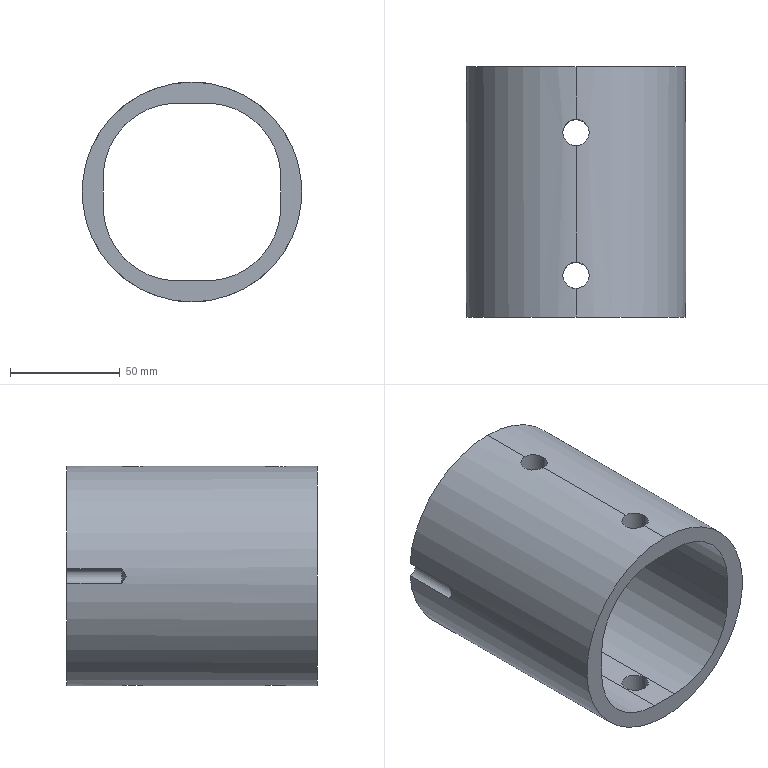Part | SolidWorks | features Extrusion 1, HoleWzd 1, ICE 1 | 1 solid | 24 faces | box 100 x 114 x 100 mm | volume 255348 mm3 | cylinder 16 | plane 6 | cone 2 | commonest cylinder face diameters 12 x8 68 x4 6.8 x2 100 x2
STEP:
#1=CARTESIAN_POINT('',(6.,-38.,40.5));
#2=VERTEX_POINT('',#1);
#3=CARTESIAN_POINT('',(-6.,-38.,40.5));
#4=VERTEX_POINT('',#3);
#5=CARTESIAN_POINT('',(0.,-38.,40.5));
#6=DIRECTION('',(0.,0.,-1.));
#7=DIRECTION('',(-1.,0.,0.));
#8=AXIS2_PLACEMENT_3D('',#5,#6,#7);
#9=CIRCLE('',#8,6.);
#10=EDGE_CURVE('',#2,#4,#9,.T.);
#11=ORIENTED_EDGE('',*,*,#10,.T.);
#12=CARTESIAN_POINT('',(-6.,-38.,49.639));
#13=VERTEX_POINT('',#12);
#14=CARTESIAN_POINT('',(-6.,-38.,-75.));
#15=DIRECTION('',(0.,0.,1.));
#16=VECTOR('',#15,1000.);
#17=LINE('',#14,#16);
#18=EDGE_CURVE('',#4,#13,#17,.T.);
#19=ORIENTED_EDGE('',*,*,#18,.T.);
#20=CARTESIAN_POINT('',(0.,-44.,50.));
#21=VERTEX_POINT('',#20);
#22=CARTESIAN_POINT('',(0.,-44.,50.));
#23=CARTESIAN_POINT('',(-0.3917,-44.,50.));
#24=CARTESIAN_POINT('',(-0.7895,-43.961,49.995));
#25=CARTESIAN_POINT('',(-1.559,-43.807,49.977));
#26=CARTESIAN_POINT('',(-1.933,-43.694,49.964));
#27=CARTESIAN_POINT('',(-2.478,-43.468,49.939));
#28=CARTESIAN_POINT('',(-2.658,-43.383,49.93));
#29=CARTESIAN_POINT('',(-3.005,-43.197,49.91));
#30=CARTESIAN_POINT('',(-3.173,-43.096,49.899));
#31=CARTESIAN_POINT('',(-3.66,-42.77,49.867));
#32=CARTESIAN_POINT('',(-3.963,-42.522,49.843));
#33=CARTESIAN_POINT('',(-4.523,-41.962,49.796));
#34=CARTESIAN_POINT('',(-4.771,-41.66,49.772));
#35=CARTESIAN_POINT('',(-5.096,-41.173,49.74));
#36=CARTESIAN_POINT('',(-5.197,-41.005,49.729));
#37=CARTESIAN_POINT('',(-5.383,-40.658,49.709));
#38=CARTESIAN_POINT('',(-5.468,-40.478,49.7));
#39=CARTESIAN_POINT('',(-5.694,-39.933,49.675));
#40=CARTESIAN_POINT('',(-5.807,-39.559,49.662));
#41=CARTESIAN_POINT('',(-5.961,-38.79,49.643));
#42=CARTESIAN_POINT('',(-6.,-38.392,49.639));
#43=CARTESIAN_POINT('',(-6.,-38.,49.639));
#44=B_SPLINE_CURVE_WITH_KNOTS('',3,(#22,#23,#24,#25,#26,#27,#28,#29,#30,#31,#32,#33,#34,#35,#36,#37,#38,#39,#40,#41,#42,#43),.UNSPECIFIED.,.F.,.F.,(4,2,2,2,2,2,2,2,2,2,4),(0.00939,0.01056,0.01174,0.01232,0.01291,0.01408,0.01526,0.01584,0.01643,0.0176,0.01878),.UNSPECIFIED.);
#45=EDGE_CURVE('',#21,#13,#44,.T.);
#46=ORIENTED_EDGE('',*,*,#45,.F.);
#47=CARTESIAN_POINT('',(6.,-38.,49.639));
#48=VERTEX_POINT('',#47);
#49=CARTESIAN_POINT('',(6.,-38.,49.639));
#50=CARTESIAN_POINT('',(6.,-38.397,49.639));
#51=CARTESIAN_POINT('',(5.961,-38.787,49.643));
#52=CARTESIAN_POINT('',(5.846,-39.363,49.657));
#53=CARTESIAN_POINT('',(5.799,-39.553,49.663));
#54=CARTESIAN_POINT('',(5.684,-39.93,49.676));
#55=CARTESIAN_POINT('',(5.617,-40.118,49.684));
#56=CARTESIAN_POINT('',(5.391,-40.663,49.709));
#57=CARTESIAN_POINT('',(5.207,-41.007,49.729));
#58=CARTESIAN_POINT('',(4.771,-41.659,49.772));
#59=CARTESIAN_POINT('',(4.518,-41.968,49.796));
#60=CARTESIAN_POINT('',(3.964,-42.521,49.843));
#61=CARTESIAN_POINT('',(3.662,-42.769,49.867));
#62=CARTESIAN_POINT('',(3.17,-43.098,49.9));
#63=CARTESIAN_POINT('',(3.,-43.2,49.91));
#64=CARTESIAN_POINT('',(2.654,-43.385,49.93));
#65=CARTESIAN_POINT('',(2.3,-43.552,49.948));
#66=CARTESIAN_POINT('',(1.931,-43.684,49.963));
#67=CARTESIAN_POINT('',(1.556,-43.798,49.976));
#68=CARTESIAN_POINT('',(1.363,-43.847,49.982));
#69=CARTESIAN_POINT('',(0.7815,-43.962,49.995));
#70=CARTESIAN_POINT('',(0.3918,-44.,50.));
#71=CARTESIAN_POINT('',(0.,-44.,50.));
#72=B_SPLINE_CURVE_WITH_KNOTS('',3,(#49,#50,#51,#52,#53,#54,#55,#56,#57,#58,#59,#60,#61,#62,#63,#64,#65,#66,#67,#68,#69,#70,#71),.UNSPECIFIED.,.F.,.F.,(4,2,2,2,2,2,2,2,1,2,2,4),(0.,0.001174,0.001761,0.002348,0.003521,0.004695,0.005869,0.006456,0.007043,0.007629,0.008216,0.00939),.UNSPECIFIED.);
#73=EDGE_CURVE('',#48,#21,#72,.T.);
#74=ORIENTED_EDGE('',*,*,#73,.F.);
#75=CARTESIAN_POINT('',(6.,-38.,-75.));
#76=DIRECTION('',(0.,0.,1.));
#77=VECTOR('',#76,1000.);
#78=LINE('',#75,#77);
#79=EDGE_CURVE('',#2,#48,#78,.T.);
#80=ORIENTED_EDGE('',*,*,#79,.F.);
#81=EDGE_LOOP('',(#11,#19,#46,#74,#80));
#82=FACE_OUTER_BOUND('',#81,.T.);
#83=CARTESIAN_POINT('',(0.,-38.,-75.));
#84=DIRECTION('',(0.,0.,1.));
#85=DIRECTION('',(1.,0.,0.));
#86=AXIS2_PLACEMENT_3D('',#83,#84,#85);
#87=CYLINDRICAL_SURFACE('',#86,6.);
#88=ADVANCED_FACE('',(#82),#87,.F.);
#89=CARTESIAN_POINT('',(6.,27.,40.5));
#90=VERTEX_POINT('',#89);
#91=CARTESIAN_POINT('',(-6.,27.,40.5));
#92=VERTEX_POINT('',#91);
#93=CARTESIAN_POINT('',(0.,27.,40.5));
#94=DIRECTION('',(0.,0.,-1.));
#95=DIRECTION('',(-1.,0.,0.));
#96=AXIS2_PLACEMENT_3D('',#93,#94,#95);
#97=CIRCLE('',#96,6.);
#98=EDGE_CURVE('',#90,#92,#97,.T.);
#99=ORIENTED_EDGE('',*,*,#98,.T.);
#100=CARTESIAN_POINT('',(-6.,27.,49.639));
#101=VERTEX_POINT('',#100);
#102=CARTESIAN_POINT('',(-6.,27.,-75.));
#103=DIRECTION('',(0.,0.,1.));
#104=VECTOR('',#103,1000.);
#105=LINE('',#102,#104);
#106=EDGE_CURVE('',#92,#101,#105,.T.);
#107=ORIENTED_EDGE('',*,*,#106,.T.);
#108=CARTESIAN_POINT('',(0.,21.,50.));
#109=VERTEX_POINT('',#108);
#110=CARTESIAN_POINT('',(0.,21.,50.));
#111=CARTESIAN_POINT('',(-0.3917,21.,50.));
#112=CARTESIAN_POINT('',(-0.7895,21.039,49.995));
#113=CARTESIAN_POINT('',(-1.559,21.193,49.977));
#114=CARTESIAN_POINT('',(-1.933,21.306,49.964));
#115=CARTESIAN_POINT('',(-2.478,21.532,49.939));
#116=CARTESIAN_POINT('',(-2.658,21.617,49.93));
#117=CARTESIAN_POINT('',(-3.005,21.803,49.91));
#118=CARTESIAN_POINT('',(-3.173,21.904,49.899));
#119=CARTESIAN_POINT('',(-3.66,22.23,49.867));
#120=CARTESIAN_POINT('',(-3.963,22.478,49.843));
#121=CARTESIAN_POINT('',(-4.523,23.038,49.796));
#122=CARTESIAN_POINT('',(-4.771,23.34,49.772));
#123=CARTESIAN_POINT('',(-5.096,23.827,49.74));
#124=CARTESIAN_POINT('',(-5.197,23.995,49.729));
#125=CARTESIAN_POINT('',(-5.383,24.342,49.709));
#126=CARTESIAN_POINT('',(-5.468,24.522,49.7));
#127=CARTESIAN_POINT('',(-5.694,25.067,49.675));
#128=CARTESIAN_POINT('',(-5.807,25.441,49.662));
#129=CARTESIAN_POINT('',(-5.961,26.21,49.643));
#130=CARTESIAN_POINT('',(-6.,26.608,49.639));
#131=CARTESIAN_POINT('',(-6.,27.,49.639));
#132=B_SPLINE_CURVE_WITH_KNOTS('',3,(#110,#111,#112,#113,#114,#115,#116,#117,#118,#119,#120,#121,#122,#123,#124,#125,#126,#127,#128,#129,#130,#131),.UNSPECIFIED.,.F.,.F.,(4,2,2,2,2,2,2,2,2,2,4),(0.00939,0.01056,0.01174,0.01232,0.01291,0.01408,0.01526,0.01584,0.01643,0.0176,0.01878),.UNSPECIFIED.);
#133=EDGE_CURVE('',#109,#101,#132,.T.);
#134=ORIENTED_EDGE('',*,*,#133,.F.);
#135=CARTESIAN_POINT('',(6.,27.,49.639));
#136=VERTEX_POINT('',#135);
#137=CARTESIAN_POINT('',(6.,27.,49.639));
#138=CARTESIAN_POINT('',(6.,26.603,49.639));
#139=CARTESIAN_POINT('',(5.961,26.213,49.643));
#140=CARTESIAN_POINT('',(5.846,25.637,49.657));
#141=CARTESIAN_POINT('',(5.799,25.447,49.663));
#142=CARTESIAN_POINT('',(5.684,25.07,49.676));
#143=CARTESIAN_POINT('',(5.617,24.882,49.684));
#144=CARTESIAN_POINT('',(5.391,24.337,49.709));
#145=CARTESIAN_POINT('',(5.207,23.993,49.729));
#146=CARTESIAN_POINT('',(4.771,23.341,49.772));
#147=CARTESIAN_POINT('',(4.518,23.032,49.796));
#148=CARTESIAN_POINT('',(3.964,22.479,49.843));
#149=CARTESIAN_POINT('',(3.662,22.231,49.867));
#150=CARTESIAN_POINT('',(3.17,21.902,49.9));
#151=CARTESIAN_POINT('',(3.,21.8,49.91));
#152=CARTESIAN_POINT('',(2.654,21.615,49.93));
#153=CARTESIAN_POINT('',(2.3,21.448,49.948));
#154=CARTESIAN_POINT('',(1.931,21.316,49.963));
#155=CARTESIAN_POINT('',(1.556,21.202,49.976));
#156=CARTESIAN_POINT('',(1.363,21.153,49.982));
#157=CARTESIAN_POINT('',(0.7815,21.038,49.995));
#158=CARTESIAN_POINT('',(0.3918,21.,50.));
#159=CARTESIAN_POINT('',(0.,21.,50.));
#160=B_SPLINE_CURVE_WITH_KNOTS('',3,(#137,#138,#139,#140,#141,#142,#143,#144,#145,#146,#147,#148,#149,#150,#151,#152,#153,#154,#155,#156,#157,#158,#159),.UNSPECIFIED.,.F.,.F.,(4,2,2,2,2,2,2,2,1,2,2,4),(0.,0.001174,0.001761,0.002348,0.003521,0.004695,0.005869,0.006456,0.007043,0.007629,0.008216,0.00939),.UNSPECIFIED.);
#161=EDGE_CURVE('',#136,#109,#160,.T.);
#162=ORIENTED_EDGE('',*,*,#161,.F.);
#163=CARTESIAN_POINT('',(6.,27.,-75.));
#164=DIRECTION('',(0.,0.,1.));
#165=VECTOR('',#164,1000.);
#166=LINE('',#163,#165);
#167=EDGE_CURVE('',#90,#136,#166,.T.);
#168=ORIENTED_EDGE('',*,*,#167,.F.);
#169=EDGE_LOOP('',(#99,#107,#134,#162,#168));
#170=FACE_OUTER_BOUND('',#169,.T.);
#171=CARTESIAN_POINT('',(0.,27.,-75.));
#172=DIRECTION('',(0.,0.,1.));
#173=DIRECTION('',(1.,0.,0.));
#174=AXIS2_PLACEMENT_3D('',#171,#172,#173);
#175=CYLINDRICAL_SURFACE('',#174,6.);
#176=ADVANCED_FACE('',(#170),#175,.F.);
#177=CARTESIAN_POINT('',(-6.,-38.,-49.639));
#178=VERTEX_POINT('',#177);
#179=CARTESIAN_POINT('',(0.,-44.,-50.));
#180=VERTEX_POINT('',#179);
#181=CARTESIAN_POINT('',(-6.,-38.,-49.639));
#182=CARTESIAN_POINT('',(-6.,-38.392,-49.639));
#183=CARTESIAN_POINT('',(-5.961,-38.789,-49.643));
#184=CARTESIAN_POINT('',(-5.807,-39.559,-49.662));
#185=CARTESIAN_POINT('',(-5.694,-39.933,-49.675));
#186=CARTESIAN_POINT('',(-5.468,-40.478,-49.7));
#187=CARTESIAN_POINT('',(-5.383,-40.658,-49.71));
#188=CARTESIAN_POINT('',(-5.197,-41.005,-49.729));
#189=CARTESIAN_POINT('',(-5.096,-41.173,-49.74));
#190=CARTESIAN_POINT('',(-4.77,-41.66,-49.772));
#191=CARTESIAN_POINT('',(-4.522,-41.963,-49.796));
#192=CARTESIAN_POINT('',(-3.962,-42.523,-49.844));
#193=CARTESIAN_POINT('',(-3.66,-42.771,-49.867));
#194=CARTESIAN_POINT('',(-3.173,-43.096,-49.9));
#195=CARTESIAN_POINT('',(-3.005,-43.197,-49.91));
#196=CARTESIAN_POINT('',(-2.658,-43.383,-49.93));
#197=CARTESIAN_POINT('',(-2.478,-43.468,-49.939));
#198=CARTESIAN_POINT('',(-1.933,-43.694,-49.964));
#199=CARTESIAN_POINT('',(-1.559,-43.807,-49.977));
#200=CARTESIAN_POINT('',(-0.7895,-43.961,-49.995));
#201=CARTESIAN_POINT('',(-0.3917,-44.,-50.));
#202=CARTESIAN_POINT('',(0.,-44.,-50.));
#203=B_SPLINE_CURVE_WITH_KNOTS('',3,(#181,#182,#183,#184,#185,#186,#187,#188,#189,#190,#191,#192,#193,#194,#195,#196,#197,#198,#199,#200,#201,#202),.UNSPECIFIED.,.F.,.F.,(4,2,2,2,2,2,2,2,2,2,4),(0.00939,0.01056,0.01174,0.01232,0.01291,0.01408,0.01526,0.01584,0.01643,0.0176,0.01878),.UNSPECIFIED.);
#204=EDGE_CURVE('',#178,#180,#203,.T.);
#205=ORIENTED_EDGE('',*,*,#204,.F.);
#206=CARTESIAN_POINT('',(-6.,-38.,-40.5));
#207=VERTEX_POINT('',#206);
#208=CARTESIAN_POINT('',(-6.,-38.,-75.));
#209=DIRECTION('',(0.,0.,1.));
#210=VECTOR('',#209,1000.);
#211=LINE('',#208,#210);
#212=EDGE_CURVE('',#178,#207,#211,.T.);
#213=ORIENTED_EDGE('',*,*,#212,.T.);
#214=CARTESIAN_POINT('',(6.,-38.,-40.5));
#215=VERTEX_POINT('',#214);
#216=CARTESIAN_POINT('',(0.,-38.,-40.5));
#217=DIRECTION('',(0.,0.,1.));
#218=DIRECTION('',(1.,0.,0.));
#219=AXIS2_PLACEMENT_3D('',#216,#217,#218);
#220=CIRCLE('',#219,6.);
#221=EDGE_CURVE('',#207,#215,#220,.T.);
#222=ORIENTED_EDGE('',*,*,#221,.T.);
#223=CARTESIAN_POINT('',(6.,-38.,-49.639));
#224=VERTEX_POINT('',#223);
#225=CARTESIAN_POINT('',(6.,-38.,-75.));
#226=DIRECTION('',(0.,0.,1.));
#227=VECTOR('',#226,1000.);
#228=LINE('',#225,#227);
#229=EDGE_CURVE('',#224,#215,#228,.T.);
#230=ORIENTED_EDGE('',*,*,#229,.F.);
#231=CARTESIAN_POINT('',(0.,-44.,-50.));
#232=CARTESIAN_POINT('',(0.3919,-44.,-50.));
#233=CARTESIAN_POINT('',(0.7816,-43.962,-49.995));
#234=CARTESIAN_POINT('',(1.363,-43.847,-49.982));
#235=CARTESIAN_POINT('',(1.556,-43.798,-49.976));
#236=CARTESIAN_POINT('',(1.932,-43.684,-49.963));
#237=CARTESIAN_POINT('',(2.3,-43.552,-49.948));
#238=CARTESIAN_POINT('',(2.654,-43.385,-49.93));
#239=CARTESIAN_POINT('',(3.,-43.2,-49.91));
#240=CARTESIAN_POINT('',(3.171,-43.098,-49.9));
#241=CARTESIAN_POINT('',(3.663,-42.769,-49.867));
#242=CARTESIAN_POINT('',(3.965,-42.521,-49.843));
#243=CARTESIAN_POINT('',(4.518,-41.967,-49.796));
#244=CARTESIAN_POINT('',(4.771,-41.659,-49.772));
#245=CARTESIAN_POINT('',(5.207,-41.007,-49.729));
#246=CARTESIAN_POINT('',(5.391,-40.663,-49.709));
#247=CARTESIAN_POINT('',(5.617,-40.117,-49.684));
#248=CARTESIAN_POINT('',(5.685,-39.93,-49.676));
#249=CARTESIAN_POINT('',(5.799,-39.553,-49.663));
#250=CARTESIAN_POINT('',(5.846,-39.363,-49.657));
#251=CARTESIAN_POINT('',(5.961,-38.787,-49.643));
#252=CARTESIAN_POINT('',(6.,-38.397,-49.639));
#253=CARTESIAN_POINT('',(6.,-38.,-49.639));
#254=B_SPLINE_CURVE_WITH_KNOTS('',3,(#231,#232,#233,#234,#235,#236,#237,#238,#239,#240,#241,#242,#243,#244,#245,#246,#247,#248,#249,#250,#251,#252,#253),.UNSPECIFIED.,.F.,.F.,(4,2,2,1,2,2,2,2,2,2,2,4),(0.01878,0.01995,0.02054,0.02112,0.02171,0.0223,0.02347,0.02464,0.02582,0.0264,0.02699,0.02817),.UNSPECIFIED.);
#255=EDGE_CURVE('',#180,#224,#254,.T.);
#256=ORIENTED_EDGE('',*,*,#255,.F.);
#257=EDGE_LOOP('',(#205,#213,#222,#230,#256));
#258=FACE_OUTER_BOUND('',#257,.T.);
#259=CARTESIAN_POINT('',(0.,-38.,-75.));
#260=DIRECTION('',(0.,0.,1.));
#261=DIRECTION('',(1.,0.,0.));
#262=AXIS2_PLACEMENT_3D('',#259,#260,#261);
#263=CYLINDRICAL_SURFACE('',#262,6.);
#264=ADVANCED_FACE('',(#258),#263,.F.);
#265=CARTESIAN_POINT('',(-6.,27.,-49.639));
#266=VERTEX_POINT('',#265);
#267=CARTESIAN_POINT('',(0.,21.,-50.));
#268=VERTEX_POINT('',#267);
#269=CARTESIAN_POINT('',(-6.,27.,-49.639));
#270=CARTESIAN_POINT('',(-6.,26.608,-49.639));
#271=CARTESIAN_POINT('',(-5.961,26.211,-49.643));
#272=CARTESIAN_POINT('',(-5.807,25.441,-49.662));
#273=CARTESIAN_POINT('',(-5.694,25.067,-49.675));
#274=CARTESIAN_POINT('',(-5.468,24.522,-49.7));
#275=CARTESIAN_POINT('',(-5.383,24.342,-49.71));
#276=CARTESIAN_POINT('',(-5.197,23.995,-49.729));
#277=CARTESIAN_POINT('',(-5.096,23.827,-49.74));
#278=CARTESIAN_POINT('',(-4.77,23.34,-49.772));
#279=CARTESIAN_POINT('',(-4.522,23.037,-49.796));
#280=CARTESIAN_POINT('',(-3.962,22.477,-49.844));
#281=CARTESIAN_POINT('',(-3.66,22.229,-49.867));
#282=CARTESIAN_POINT('',(-3.173,21.904,-49.9));
#283=CARTESIAN_POINT('',(-3.005,21.803,-49.91));
#284=CARTESIAN_POINT('',(-2.658,21.617,-49.93));
#285=CARTESIAN_POINT('',(-2.478,21.532,-49.939));
#286=CARTESIAN_POINT('',(-1.933,21.306,-49.964));
#287=CARTESIAN_POINT('',(-1.559,21.193,-49.977));
#288=CARTESIAN_POINT('',(-0.7895,21.039,-49.995));
#289=CARTESIAN_POINT('',(-0.3917,21.,-50.));
#290=CARTESIAN_POINT('',(0.,21.,-50.));
#291=B_SPLINE_CURVE_WITH_KNOTS('',3,(#269,#270,#271,#272,#273,#274,#275,#276,#277,#278,#279,#280,#281,#282,#283,#284,#285,#286,#287,#288,#289,#290),.UNSPECIFIED.,.F.,.F.,(4,2,2,2,2,2,2,2,2,2,4),(0.00939,0.01056,0.01174,0.01232,0.01291,0.01408,0.01526,0.01584,0.01643,0.0176,0.01878),.UNSPECIFIED.);
#292=EDGE_CURVE('',#266,#268,#291,.T.);
#293=ORIENTED_EDGE('',*,*,#292,.F.);
#294=CARTESIAN_POINT('',(-6.,27.,-40.5));
#295=VERTEX_POINT('',#294);
#296=CARTESIAN_POINT('',(-6.,27.,-75.));
#297=DIRECTION('',(0.,0.,1.));
#298=VECTOR('',#297,1000.);
#299=LINE('',#296,#298);
#300=EDGE_CURVE('',#266,#295,#299,.T.);
#301=ORIENTED_EDGE('',*,*,#300,.T.);
#302=CARTESIAN_POINT('',(6.,27.,-40.5));
#303=VERTEX_POINT('',#302);
#304=CARTESIAN_POINT('',(0.,27.,-40.5));
#305=DIRECTION('',(0.,0.,1.));
#306=DIRECTION('',(1.,0.,0.));
#307=AXIS2_PLACEMENT_3D('',#304,#305,#306);
#308=CIRCLE('',#307,6.);
#309=EDGE_CURVE('',#295,#303,#308,.T.);
#310=ORIENTED_EDGE('',*,*,#309,.T.);
#311=CARTESIAN_POINT('',(6.,27.,-49.639));
#312=VERTEX_POINT('',#311);
#313=CARTESIAN_POINT('',(6.,27.,-75.));
#314=DIRECTION('',(0.,0.,1.));
#315=VECTOR('',#314,1000.);
#316=LINE('',#313,#315);
#317=EDGE_CURVE('',#312,#303,#316,.T.);
#318=ORIENTED_EDGE('',*,*,#317,.F.);
#319=CARTESIAN_POINT('',(0.,21.,-50.));
#320=CARTESIAN_POINT('',(0.3919,21.,-50.));
#321=CARTESIAN_POINT('',(0.7816,21.038,-49.995));
#322=CARTESIAN_POINT('',(1.363,21.153,-49.982));
#323=CARTESIAN_POINT('',(1.556,21.202,-49.976));
#324=CARTESIAN_POINT('',(1.932,21.316,-49.963));
#325=CARTESIAN_POINT('',(2.3,21.448,-49.948));
#326=CARTESIAN_POINT('',(2.654,21.615,-49.93));
#327=CARTESIAN_POINT('',(3.,21.8,-49.91));
#328=CARTESIAN_POINT('',(3.171,21.902,-49.9));
#329=CARTESIAN_POINT('',(3.663,22.231,-49.867));
#330=CARTESIAN_POINT('',(3.965,22.479,-49.843));
#331=CARTESIAN_POINT('',(4.518,23.033,-49.796));
#332=CARTESIAN_POINT('',(4.771,23.341,-49.772));
#333=CARTESIAN_POINT('',(5.207,23.993,-49.729));
#334=CARTESIAN_POINT('',(5.391,24.337,-49.709));
#335=CARTESIAN_POINT('',(5.617,24.883,-49.684));
#336=CARTESIAN_POINT('',(5.685,25.07,-49.676));
#337=CARTESIAN_POINT('',(5.799,25.447,-49.663));
#338=CARTESIAN_POINT('',(5.846,25.637,-49.657));
#339=CARTESIAN_POINT('',(5.961,26.213,-49.643));
#340=CARTESIAN_POINT('',(6.,26.603,-49.639));
#341=CARTESIAN_POINT('',(6.,27.,-49.639));
#342=B_SPLINE_CURVE_WITH_KNOTS('',3,(#319,#320,#321,#322,#323,#324,#325,#326,#327,#328,#329,#330,#331,#332,#333,#334,#335,#336,#337,#338,#339,#340,#341),.UNSPECIFIED.,.F.,.F.,(4,2,2,1,2,2,2,2,2,2,2,4),(0.01878,0.01995,0.02054,0.02112,0.02171,0.0223,0.02347,0.02464,0.02582,0.0264,0.02699,0.02817),.UNSPECIFIED.);
#343=EDGE_CURVE('',#268,#312,#342,.T.);
#344=ORIENTED_EDGE('',*,*,#343,.F.);
#345=EDGE_LOOP('',(#293,#301,#310,#318,#344));
#346=FACE_OUTER_BOUND('',#345,.T.);
#347=CARTESIAN_POINT('',(0.,27.,-75.));
#348=DIRECTION('',(0.,0.,1.));
#349=DIRECTION('',(1.,0.,0.));
#350=AXIS2_PLACEMENT_3D('',#347,#348,#349);
#351=CYLINDRICAL_SURFACE('',#350,6.);
#352=ADVANCED_FACE('',(#346),#351,.F.);
#353=CARTESIAN_POINT('',(0.,57.,50.));
#354=VERTEX_POINT('',#353);
#355=CARTESIAN_POINT('',(49.884,57.,3.398));
#356=VERTEX_POINT('',#355);
#357=CARTESIAN_POINT('',(0.,57.,0.));
#358=DIRECTION('',(0.,1.,0.));
#359=DIRECTION('',(0.,0.,1.));
#360=AXIS2_PLACEMENT_3D('',#357,#358,#359);
#361=CIRCLE('',#360,50.);
#362=EDGE_CURVE('',#354,#356,#361,.T.);
#363=ORIENTED_EDGE('',*,*,#362,.F.);
#364=CARTESIAN_POINT('',(0.,33.,50.));
#365=VERTEX_POINT('',#364);
#366=CARTESIAN_POINT('',(0.,57.,50.));
#367=DIRECTION('',(0.,-1.,0.));
#368=VECTOR('',#367,1000.);
#369=LINE('',#366,#368);
#370=EDGE_CURVE('',#354,#365,#369,.T.);
#371=ORIENTED_EDGE('',*,*,#370,.T.);
#372=CARTESIAN_POINT('',(0.,33.,50.));
#373=CARTESIAN_POINT('',(0.3965,33.,50.));
#374=CARTESIAN_POINT('',(0.7864,32.961,49.995));
#375=CARTESIAN_POINT('',(1.362,32.847,49.982));
#376=CARTESIAN_POINT('',(1.552,32.799,49.976));
#377=CARTESIAN_POINT('',(1.929,32.685,49.963));
#378=CARTESIAN_POINT('',(2.116,32.618,49.956));
#379=CARTESIAN_POINT('',(2.66,32.392,49.93));
#380=CARTESIAN_POINT('',(3.005,32.208,49.911));
#381=CARTESIAN_POINT('',(3.657,31.773,49.867));
#382=CARTESIAN_POINT('',(3.965,31.52,49.843));
#383=CARTESIAN_POINT('',(4.518,30.968,49.796));
#384=CARTESIAN_POINT('',(4.766,30.666,49.773));
#385=CARTESIAN_POINT('',(5.095,30.175,49.74));
#386=CARTESIAN_POINT('',(5.197,30.005,49.729));
#387=CARTESIAN_POINT('',(5.382,29.659,49.71));
#388=CARTESIAN_POINT('',(5.466,29.483,49.7));
#389=CARTESIAN_POINT('',(5.691,28.942,49.675));
#390=CARTESIAN_POINT('',(5.806,28.564,49.662));
#391=CARTESIAN_POINT('',(5.961,27.789,49.643));
#392=CARTESIAN_POINT('',(6.,27.397,49.639));
#393=CARTESIAN_POINT('',(6.,27.,49.639));
#394=B_SPLINE_CURVE_WITH_KNOTS('',3,(#372,#373,#374,#375,#376,#377,#378,#379,#380,#381,#382,#383,#384,#385,#386,#387,#388,#389,#390,#391,#392,#393),.UNSPECIFIED.,.F.,.F.,(4,2,2,2,2,2,2,2,2,2,4),(0.02817,0.02934,0.02992,0.03051,0.03168,0.03286,0.03403,0.03462,0.0352,0.03637,0.03755),.UNSPECIFIED.);
#395=EDGE_CURVE('',#365,#136,#394,.T.);
#396=ORIENTED_EDGE('',*,*,#395,.T.);
#397=ORIENTED_EDGE('',*,*,#161,.T.);
#398=CARTESIAN_POINT('',(0.,-32.,50.));
#399=VERTEX_POINT('',#398);
#400=CARTESIAN_POINT('',(0.,57.,50.));
#401=DIRECTION('',(0.,-1.,0.));
#402=VECTOR('',#401,1000.);
#403=LINE('',#400,#402);
#404=EDGE_CURVE('',#109,#399,#403,.T.);
#405=ORIENTED_EDGE('',*,*,#404,.T.);
#406=CARTESIAN_POINT('',(0.,-32.,50.));
#407=CARTESIAN_POINT('',(0.3965,-32.,50.));
#408=CARTESIAN_POINT('',(0.7864,-32.039,49.995));
#409=CARTESIAN_POINT('',(1.362,-32.153,49.982));
#410=CARTESIAN_POINT('',(1.552,-32.201,49.976));
#411=CARTESIAN_POINT('',(1.929,-32.315,49.963));
#412=CARTESIAN_POINT('',(2.116,-32.382,49.956));
#413=CARTESIAN_POINT('',(2.66,-32.608,49.93));
#414=CARTESIAN_POINT('',(3.005,-32.792,49.911));
#415=CARTESIAN_POINT('',(3.657,-33.227,49.867));
#416=CARTESIAN_POINT('',(3.965,-33.48,49.843));
#417=CARTESIAN_POINT('',(4.518,-34.032,49.796));
#418=CARTESIAN_POINT('',(4.766,-34.334,49.773));
#419=CARTESIAN_POINT('',(5.095,-34.825,49.74));
#420=CARTESIAN_POINT('',(5.197,-34.995,49.729));
#421=CARTESIAN_POINT('',(5.382,-35.341,49.71));
#422=CARTESIAN_POINT('',(5.466,-35.517,49.7));
#423=CARTESIAN_POINT('',(5.691,-36.058,49.675));
#424=CARTESIAN_POINT('',(5.806,-36.436,49.662));
#425=CARTESIAN_POINT('',(5.961,-37.211,49.643));
#426=CARTESIAN_POINT('',(6.,-37.603,49.639));
#427=CARTESIAN_POINT('',(6.,-38.,49.639));
#428=B_SPLINE_CURVE_WITH_KNOTS('',3,(#406,#407,#408,#409,#410,#411,#412,#413,#414,#415,#416,#417,#418,#419,#420,#421,#422,#423,#424,#425,#426,#427),.UNSPECIFIED.,.F.,.F.,(4,2,2,2,2,2,2,2,2,2,4),(0.02817,0.02934,0.02992,0.03051,0.03168,0.03286,0.03403,0.03462,0.0352,0.03637,0.03755),.UNSPECIFIED.);
#429=EDGE_CURVE('',#399,#48,#428,.T.);
#430=ORIENTED_EDGE('',*,*,#429,.T.);
#431=ORIENTED_EDGE('',*,*,#73,.T.);
#432=CARTESIAN_POINT('',(0.,-57.,50.));
#433=VERTEX_POINT('',#432);
#434=CARTESIAN_POINT('',(0.,57.,50.));
#435=DIRECTION('',(0.,-1.,0.));
#436=VECTOR('',#435,1000.);
#437=LINE('',#434,#436);
#438=EDGE_CURVE('',#21,#433,#437,.T.);
#439=ORIENTED_EDGE('',*,*,#438,.T.);
#440=CARTESIAN_POINT('',(0.,-57.,-50.));
#441=VERTEX_POINT('',#440);
#442=CARTESIAN_POINT('',(0.,-57.,0.));
#443=DIRECTION('',(0.,1.,0.));
#444=DIRECTION('',(0.,0.,1.));
#445=AXIS2_PLACEMENT_3D('',#442,#443,#444);
#446=CIRCLE('',#445,50.);
#447=EDGE_CURVE('',#433,#441,#446,.T.);
#448=ORIENTED_EDGE('',*,*,#447,.T.);
#449=CARTESIAN_POINT('',(0.,57.,-50.));
#450=DIRECTION('',(0.,-1.,0.));
#451=VECTOR('',#450,1000.);
#452=LINE('',#449,#451);
#453=EDGE_CURVE('',#180,#441,#452,.T.);
#454=ORIENTED_EDGE('',*,*,#453,.F.);
#455=ORIENTED_EDGE('',*,*,#255,.T.);
#456=CARTESIAN_POINT('',(0.,-32.,-50.));
#457=VERTEX_POINT('',#456);
#458=CARTESIAN_POINT('',(6.,-38.,-49.639));
#459=CARTESIAN_POINT('',(6.,-37.603,-49.639));
#460=CARTESIAN_POINT('',(5.961,-37.214,-49.643));
#461=CARTESIAN_POINT('',(5.847,-36.638,-49.657));
#462=CARTESIAN_POINT('',(5.799,-36.448,-49.663));
#463=CARTESIAN_POINT('',(5.685,-36.071,-49.676));
#464=CARTESIAN_POINT('',(5.618,-35.884,-49.683));
#465=CARTESIAN_POINT('',(5.392,-35.34,-49.709));
#466=CARTESIAN_POINT('',(5.208,-34.995,-49.728));
#467=CARTESIAN_POINT('',(4.773,-34.343,-49.772));
#468=CARTESIAN_POINT('',(4.52,-34.035,-49.796));
#469=CARTESIAN_POINT('',(3.968,-33.482,-49.843));
#470=CARTESIAN_POINT('',(3.666,-33.234,-49.866));
#471=CARTESIAN_POINT('',(3.175,-32.905,-49.899));
#472=CARTESIAN_POINT('',(3.005,-32.803,-49.91));
#473=CARTESIAN_POINT('',(2.659,-32.618,-49.93));
#474=CARTESIAN_POINT('',(2.483,-32.534,-49.939));
#475=CARTESIAN_POINT('',(1.942,-32.309,-49.964));
#476=CARTESIAN_POINT('',(1.564,-32.194,-49.977));
#477=CARTESIAN_POINT('',(0.7886,-32.039,-49.995));
#478=CARTESIAN_POINT('',(0.3965,-32.,-50.));
#479=CARTESIAN_POINT('',(0.,-32.,-50.));
#480=B_SPLINE_CURVE_WITH_KNOTS('',3,(#458,#459,#460,#461,#462,#463,#464,#465,#466,#467,#468,#469,#470,#471,#472,#473,#474,#475,#476,#477,#478,#479),.UNSPECIFIED.,.F.,.F.,(4,2,2,2,2,2,2,2,2,2,4),(0.02817,0.02934,0.02992,0.03051,0.03168,0.03286,0.03403,0.03462,0.0352,0.03637,0.03755),.UNSPECIFIED.);
#481=EDGE_CURVE('',#224,#457,#480,.T.);
#482=ORIENTED_EDGE('',*,*,#481,.T.);
#483=CARTESIAN_POINT('',(0.,57.,-50.));
#484=DIRECTION('',(0.,-1.,0.));
#485=VECTOR('',#484,1000.);
#486=LINE('',#483,#485);
#487=EDGE_CURVE('',#268,#457,#486,.T.);
#488=ORIENTED_EDGE('',*,*,#487,.F.);
#489=ORIENTED_EDGE('',*,*,#343,.T.);
#490=CARTESIAN_POINT('',(0.,33.,-50.));
#491=VERTEX_POINT('',#490);
#492=CARTESIAN_POINT('',(6.,27.,-49.639));
#493=CARTESIAN_POINT('',(6.,27.397,-49.639));
#494=CARTESIAN_POINT('',(5.961,27.786,-49.643));
#495=CARTESIAN_POINT('',(5.847,28.362,-49.657));
#496=CARTESIAN_POINT('',(5.799,28.552,-49.663));
#497=CARTESIAN_POINT('',(5.685,28.929,-49.676));
#498=CARTESIAN_POINT('',(5.618,29.116,-49.683));
#499=CARTESIAN_POINT('',(5.392,29.66,-49.709));
#500=CARTESIAN_POINT('',(5.208,30.005,-49.728));
#501=CARTESIAN_POINT('',(4.773,30.657,-49.772));
#502=CARTESIAN_POINT('',(4.52,30.965,-49.796));
#503=CARTESIAN_POINT('',(3.968,31.518,-49.843));
#504=CARTESIAN_POINT('',(3.666,31.766,-49.866));
#505=CARTESIAN_POINT('',(3.175,32.095,-49.899));
#506=CARTESIAN_POINT('',(3.005,32.197,-49.91));
#507=CARTESIAN_POINT('',(2.659,32.382,-49.93));
#508=CARTESIAN_POINT('',(2.483,32.466,-49.939));
#509=CARTESIAN_POINT('',(1.942,32.691,-49.964));
#510=CARTESIAN_POINT('',(1.564,32.806,-49.977));
#511=CARTESIAN_POINT('',(0.7886,32.961,-49.995));
#512=CARTESIAN_POINT('',(0.3965,33.,-50.));
#513=CARTESIAN_POINT('',(0.,33.,-50.));
#514=B_SPLINE_CURVE_WITH_KNOTS('',3,(#492,#493,#494,#495,#496,#497,#498,#499,#500,#501,#502,#503,#504,#505,#506,#507,#508,#509,#510,#511,#512,#513),.UNSPECIFIED.,.F.,.F.,(4,2,2,2,2,2,2,2,2,2,4),(0.02817,0.02934,0.02992,0.03051,0.03168,0.03286,0.03403,0.03462,0.0352,0.03637,0.03755),.UNSPECIFIED.);
#515=EDGE_CURVE('',#312,#491,#514,.T.);
#516=ORIENTED_EDGE('',*,*,#515,.T.);
#517=CARTESIAN_POINT('',(0.,57.,-50.));
#518=VERTEX_POINT('',#517);
#519=CARTESIAN_POINT('',(0.,57.,-50.));
#520=DIRECTION('',(0.,-1.,0.));
#521=VECTOR('',#520,1000.);
#522=LINE('',#519,#521);
#523=EDGE_CURVE('',#518,#491,#522,.T.);
#524=ORIENTED_EDGE('',*,*,#523,.F.);
#525=CARTESIAN_POINT('',(49.884,57.,-3.398));
#526=VERTEX_POINT('',#525);
#527=CARTESIAN_POINT('',(0.,57.,0.));
#528=DIRECTION('',(0.,1.,0.));
#529=DIRECTION('',(0.,0.,1.));
#530=AXIS2_PLACEMENT_3D('',#527,#528,#529);
#531=CIRCLE('',#530,50.);
#532=EDGE_CURVE('',#526,#518,#531,.T.);
#533=ORIENTED_EDGE('',*,*,#532,.F.);
#534=CARTESIAN_POINT('',(49.884,32.,-3.398));
#535=VERTEX_POINT('',#534);
#536=CARTESIAN_POINT('',(49.884,44.5,-3.398));
#537=DIRECTION('',(0.,-1.,0.));
#538=VECTOR('',#537,1000.);
#539=LINE('',#536,#538);
#540=EDGE_CURVE('',#526,#535,#539,.T.);
#541=ORIENTED_EDGE('',*,*,#540,.T.);
#542=CARTESIAN_POINT('',(50.,29.957,0.));
#543=VERTEX_POINT('',#542);
#544=CARTESIAN_POINT('',(49.884,32.,-3.398));
#545=CARTESIAN_POINT('',(49.961,31.319,-2.267));
#546=CARTESIAN_POINT('',(50.,30.638,-1.133));
#547=CARTESIAN_POINT('',(50.,29.957,0.));
#548=B_SPLINE_CURVE_WITH_KNOTS('',3,(#544,#545,#546,#547),.UNSPECIFIED.,.F.,.F.,(4,4),(0.0004031,0.00437),.UNSPECIFIED.);
#549=EDGE_CURVE('',#535,#543,#548,.T.);
#550=ORIENTED_EDGE('',*,*,#549,.T.);
#551=CARTESIAN_POINT('',(49.884,32.,3.398));
#552=VERTEX_POINT('',#551);
#553=CARTESIAN_POINT('',(50.,29.957,0.));
#554=CARTESIAN_POINT('',(50.,30.638,1.134));
#555=CARTESIAN_POINT('',(49.961,31.319,2.267));
#556=CARTESIAN_POINT('',(49.884,32.,3.398));
#557=B_SPLINE_CURVE_WITH_KNOTS('',3,(#553,#554,#555,#556),.UNSPECIFIED.,.F.,.F.,(4,4),(-0.000000022,0.003968),.UNSPECIFIED.);
#558=EDGE_CURVE('',#543,#552,#557,.T.);
#559=ORIENTED_EDGE('',*,*,#558,.T.);
#560=CARTESIAN_POINT('',(49.884,44.5,3.398));
#561=DIRECTION('',(0.,1.,0.));
#562=VECTOR('',#561,1000.);
#563=LINE('',#560,#562);
#564=EDGE_CURVE('',#552,#356,#563,.T.);
#565=ORIENTED_EDGE('',*,*,#564,.T.);
#566=EDGE_LOOP('',(#363,#371,#396,#397,#405,#430,#431,#439,#448,#454,#455,#482,#488,#489,#516,#524,#533,#541,#550,#559,#565));
#567=FACE_OUTER_BOUND('',#566,.T.);
#568=CARTESIAN_POINT('',(0.,57.,0.));
#569=DIRECTION('',(0.,-1.,0.));
#570=DIRECTION('',(0.,0.,-1.));
#571=AXIS2_PLACEMENT_3D('',#568,#569,#570);
#572=CYLINDRICAL_SURFACE('',#571,50.);
#573=ADVANCED_FACE('',(#567),#572,.T.);
#574=CARTESIAN_POINT('',(-49.884,57.,3.398));
#575=VERTEX_POINT('',#574);
#576=CARTESIAN_POINT('',(-49.884,57.,-3.398));
#577=VERTEX_POINT('',#576);
#578=CARTESIAN_POINT('',(-50.,57.,0.));
#579=DIRECTION('',(0.,1.,0.));
#580=DIRECTION('',(0.,0.,1.));
#581=AXIS2_PLACEMENT_3D('',#578,#579,#580);
#582=CIRCLE('',#581,3.4);
#583=EDGE_CURVE('',#575,#577,#582,.T.);
#584=ORIENTED_EDGE('',*,*,#583,.F.);
#585=CARTESIAN_POINT('',(0.,57.,0.));
#586=DIRECTION('',(0.,1.,0.));
#587=DIRECTION('',(0.,0.,1.));
#588=AXIS2_PLACEMENT_3D('',#585,#586,#587);
#589=CIRCLE('',#588,50.);
#590=EDGE_CURVE('',#575,#354,#589,.T.);
#591=ORIENTED_EDGE('',*,*,#590,.T.);
#592=ORIENTED_EDGE('',*,*,#362,.T.);
#593=CARTESIAN_POINT('',(50.,57.,0.));
#594=DIRECTION('',(0.,1.,0.));
#595=DIRECTION('',(0.,0.,1.));
#596=AXIS2_PLACEMENT_3D('',#593,#594,#595);
#597=CIRCLE('',#596,3.4);
#598=EDGE_CURVE('',#526,#356,#597,.T.);
#599=ORIENTED_EDGE('',*,*,#598,.F.);
#600=ORIENTED_EDGE('',*,*,#532,.T.);
#601=CARTESIAN_POINT('',(0.,57.,0.));
#602=DIRECTION('',(0.,1.,0.));
#603=DIRECTION('',(0.,0.,1.));
#604=AXIS2_PLACEMENT_3D('',#601,#602,#603);
#605=CIRCLE('',#604,50.);
#606=EDGE_CURVE('',#518,#577,#605,.T.);
#607=ORIENTED_EDGE('',*,*,#606,.T.);
#608=EDGE_LOOP('',(#584,#591,#592,#599,#600,#607));
#609=FACE_OUTER_BOUND('',#608,.T.);
#610=CARTESIAN_POINT('',(-6.5,57.,40.5));
#611=VERTEX_POINT('',#610);
#612=CARTESIAN_POINT('',(6.5,57.,40.5));
#613=VERTEX_POINT('',#612);
#614=CARTESIAN_POINT('',(-6.5,57.,40.5));
#615=DIRECTION('',(1.,0.,0.));
#616=VECTOR('',#615,1000.);
#617=LINE('',#614,#616);
#618=EDGE_CURVE('',#611,#613,#617,.T.);
#619=ORIENTED_EDGE('',*,*,#618,.F.);
#620=CARTESIAN_POINT('',(-40.5,57.,6.5));
#621=VERTEX_POINT('',#620);
#622=CARTESIAN_POINT('',(-6.5,57.,6.5));
#623=DIRECTION('',(0.,1.,0.));
#624=DIRECTION('',(0.,0.,-1.));
#625=AXIS2_PLACEMENT_3D('',#622,#623,#624);
#626=CIRCLE('',#625,34.);
#627=EDGE_CURVE('',#621,#611,#626,.T.);
#628=ORIENTED_EDGE('',*,*,#627,.F.);
#629=CARTESIAN_POINT('',(-40.5,57.,-6.5));
#630=VERTEX_POINT('',#629);
#631=CARTESIAN_POINT('',(-40.5,57.,6.5));
#632=DIRECTION('',(0.,0.,1.));
#633=VECTOR('',#632,1000.);
#634=LINE('',#631,#633);
#635=EDGE_CURVE('',#630,#621,#634,.T.);
#636=ORIENTED_EDGE('',*,*,#635,.F.);
#637=CARTESIAN_POINT('',(-6.5,57.,-40.5));
#638=VERTEX_POINT('',#637);
#639=CARTESIAN_POINT('',(-6.5,57.,-6.5));
#640=DIRECTION('',(0.,1.,0.));
#641=DIRECTION('',(0.,0.,-1.));
#642=AXIS2_PLACEMENT_3D('',#639,#640,#641);
#643=CIRCLE('',#642,34.);
#644=EDGE_CURVE('',#638,#630,#643,.T.);
#645=ORIENTED_EDGE('',*,*,#644,.F.);
#646=CARTESIAN_POINT('',(6.5,57.,-40.5));
#647=VERTEX_POINT('',#646);
#648=CARTESIAN_POINT('',(-6.5,57.,-40.5));
#649=DIRECTION('',(-1.,0.,0.));
#650=VECTOR('',#649,1000.);
#651=LINE('',#648,#650);
#652=EDGE_CURVE('',#647,#638,#651,.T.);
#653=ORIENTED_EDGE('',*,*,#652,.F.);
#654=CARTESIAN_POINT('',(40.5,57.,-6.5));
#655=VERTEX_POINT('',#654);
#656=CARTESIAN_POINT('',(6.5,57.,-6.5));
#657=DIRECTION('',(0.,1.,0.));
#658=DIRECTION('',(0.,0.,-1.));
#659=AXIS2_PLACEMENT_3D('',#656,#657,#658);
#660=CIRCLE('',#659,34.);
#661=EDGE_CURVE('',#655,#647,#660,.T.);
#662=ORIENTED_EDGE('',*,*,#661,.F.);
#663=CARTESIAN_POINT('',(40.5,57.,6.5));
#664=VERTEX_POINT('',#663);
#665=CARTESIAN_POINT('',(40.5,57.,6.5));
#666=DIRECTION('',(0.,0.,-1.));
#667=VECTOR('',#666,1000.);
#668=LINE('',#665,#667);
#669=EDGE_CURVE('',#664,#655,#668,.T.);
#670=ORIENTED_EDGE('',*,*,#669,.F.);
#671=CARTESIAN_POINT('',(6.5,57.,6.5));
#672=DIRECTION('',(0.,1.,0.));
#673=DIRECTION('',(0.,0.,1.));
#674=AXIS2_PLACEMENT_3D('',#671,#672,#673);
#675=CIRCLE('',#674,34.);
#676=EDGE_CURVE('',#613,#664,#675,.T.);
#677=ORIENTED_EDGE('',*,*,#676,.F.);
#678=EDGE_LOOP('',(#619,#628,#636,#645,#653,#662,#670,#677));
#679=FACE_BOUND('',#678,.T.);
#680=CARTESIAN_POINT('',(0.,57.,0.));
#681=DIRECTION('',(0.,1.,0.));
#682=DIRECTION('',(0.,0.,1.));
#683=AXIS2_PLACEMENT_3D('',#680,#681,#682);
#684=PLANE('',#683);
#685=ADVANCED_FACE('',(#609,#679),#684,.T.);
#686=CARTESIAN_POINT('',(0.,-57.,0.));
#687=DIRECTION('',(0.,1.,0.));
#688=DIRECTION('',(0.,0.,1.));
#689=AXIS2_PLACEMENT_3D('',#686,#687,#688);
#690=CIRCLE('',#689,50.);
#691=EDGE_CURVE('',#441,#433,#690,.T.);
#692=ORIENTED_EDGE('',*,*,#691,.F.);
#693=ORIENTED_EDGE('',*,*,#447,.F.);
#694=EDGE_LOOP('',(#692,#693));
#695=FACE_OUTER_BOUND('',#694,.T.);
#696=CARTESIAN_POINT('',(-40.5,-57.,6.5));
#697=VERTEX_POINT('',#696);
#698=CARTESIAN_POINT('',(-6.5,-57.,40.5));
#699=VERTEX_POINT('',#698);
#700=CARTESIAN_POINT('',(-6.5,-57.,6.5));
#701=DIRECTION('',(0.,1.,0.));
#702=DIRECTION('',(0.,0.,-1.));
#703=AXIS2_PLACEMENT_3D('',#700,#701,#702);
#704=CIRCLE('',#703,34.);
#705=EDGE_CURVE('',#697,#699,#704,.T.);
#706=ORIENTED_EDGE('',*,*,#705,.T.);
#707=CARTESIAN_POINT('',(6.5,-57.,40.5));
#708=VERTEX_POINT('',#707);
#709=CARTESIAN_POINT('',(-6.5,-57.,40.5));
#710=DIRECTION('',(1.,0.,0.));
#711=VECTOR('',#710,1000.);
#712=LINE('',#709,#711);
#713=EDGE_CURVE('',#699,#708,#712,.T.);
#714=ORIENTED_EDGE('',*,*,#713,.T.);
#715=CARTESIAN_POINT('',(40.5,-57.,6.5));
#716=VERTEX_POINT('',#715);
#717=CARTESIAN_POINT('',(6.5,-57.,6.5));
#718=DIRECTION('',(0.,1.,0.));
#719=DIRECTION('',(0.,0.,1.));
#720=AXIS2_PLACEMENT_3D('',#717,#718,#719);
#721=CIRCLE('',#720,34.);
#722=EDGE_CURVE('',#708,#716,#721,.T.);
#723=ORIENTED_EDGE('',*,*,#722,.T.);
#724=CARTESIAN_POINT('',(40.5,-57.,-6.5));
#725=VERTEX_POINT('',#724);
#726=CARTESIAN_POINT('',(40.5,-57.,6.5));
#727=DIRECTION('',(0.,0.,-1.));
#728=VECTOR('',#727,1000.);
#729=LINE('',#726,#728);
#730=EDGE_CURVE('',#716,#725,#729,.T.);
#731=ORIENTED_EDGE('',*,*,#730,.T.);
#732=CARTESIAN_POINT('',(6.5,-57.,-40.5));
#733=VERTEX_POINT('',#732);
#734=CARTESIAN_POINT('',(6.5,-57.,-6.5));
#735=DIRECTION('',(0.,1.,0.));
#736=DIRECTION('',(0.,0.,-1.));
#737=AXIS2_PLACEMENT_3D('',#734,#735,#736);
#738=CIRCLE('',#737,34.);
#739=EDGE_CURVE('',#725,#733,#738,.T.);
#740=ORIENTED_EDGE('',*,*,#739,.T.);
#741=CARTESIAN_POINT('',(-6.5,-57.,-40.5));
#742=VERTEX_POINT('',#741);
#743=CARTESIAN_POINT('',(-6.5,-57.,-40.5));
#744=DIRECTION('',(-1.,0.,0.));
#745=VECTOR('',#744,1000.);
#746=LINE('',#743,#745);
#747=EDGE_CURVE('',#733,#742,#746,.T.);
#748=ORIENTED_EDGE('',*,*,#747,.T.);
#749=CARTESIAN_POINT('',(-40.5,-57.,-6.5));
#750=VERTEX_POINT('',#749);
#751=CARTESIAN_POINT('',(-6.5,-57.,-6.5));
#752=DIRECTION('',(0.,1.,0.));
#753=DIRECTION('',(0.,0.,-1.));
#754=AXIS2_PLACEMENT_3D('',#751,#752,#753);
#755=CIRCLE('',#754,34.);
#756=EDGE_CURVE('',#742,#750,#755,.T.);
#757=ORIENTED_EDGE('',*,*,#756,.T.);
#758=CARTESIAN_POINT('',(-40.5,-57.,6.5));
#759=DIRECTION('',(0.,0.,1.));
#760=VECTOR('',#759,1000.);
#761=LINE('',#758,#760);
#762=EDGE_CURVE('',#750,#697,#761,.T.);
#763=ORIENTED_EDGE('',*,*,#762,.T.);
#764=EDGE_LOOP('',(#706,#714,#723,#731,#740,#748,#757,#763));
#765=FACE_BOUND('',#764,.T.);
#766=CARTESIAN_POINT('',(0.,-57.,0.));
#767=DIRECTION('',(0.,1.,0.));
#768=DIRECTION('',(0.,0.,1.));
#769=AXIS2_PLACEMENT_3D('',#766,#767,#768);
#770=PLANE('',#769);
#771=ADVANCED_FACE('',(#695,#765),#770,.F.);
#772=ORIENTED_EDGE('',*,*,#370,.F.);
#773=ORIENTED_EDGE('',*,*,#590,.F.);
#774=CARTESIAN_POINT('',(-49.884,32.,3.398));
#775=VERTEX_POINT('',#774);
#776=CARTESIAN_POINT('',(-49.884,44.5,3.398));
#777=DIRECTION('',(0.,-1.,0.));
#778=VECTOR('',#777,1000.);
#779=LINE('',#776,#778);
#780=EDGE_CURVE('',#575,#775,#779,.T.);
#781=ORIENTED_EDGE('',*,*,#780,.T.);
#782=CARTESIAN_POINT('',(-50.,29.957,0.));
#783=VERTEX_POINT('',#782);
#784=CARTESIAN_POINT('',(-49.884,32.,3.398));
#785=CARTESIAN_POINT('',(-49.961,31.319,2.267));
#786=CARTESIAN_POINT('',(-50.,30.638,1.133));
#787=CARTESIAN_POINT('',(-50.,29.957,0.));
#788=B_SPLINE_CURVE_WITH_KNOTS('',3,(#784,#785,#786,#787),.UNSPECIFIED.,.F.,.F.,(4,4),(0.0004031,0.00437),.UNSPECIFIED.);
#789=EDGE_CURVE('',#775,#783,#788,.T.);
#790=ORIENTED_EDGE('',*,*,#789,.T.);
#791=CARTESIAN_POINT('',(-49.884,32.,-3.398));
#792=VERTEX_POINT('',#791);
#793=CARTESIAN_POINT('',(-50.,29.957,0.));
#794=CARTESIAN_POINT('',(-50.,30.638,-1.134));
#795=CARTESIAN_POINT('',(-49.961,31.319,-2.267));
#796=CARTESIAN_POINT('',(-49.884,32.,-3.398));
#797=B_SPLINE_CURVE_WITH_KNOTS('',3,(#793,#794,#795,#796),.UNSPECIFIED.,.F.,.F.,(4,4),(-0.000000022,0.003968),.UNSPECIFIED.);
#798=EDGE_CURVE('',#783,#792,#797,.T.);
#799=ORIENTED_EDGE('',*,*,#798,.T.);
#800=CARTESIAN_POINT('',(-49.884,44.5,-3.398));
#801=DIRECTION('',(0.,1.,0.));
#802=VECTOR('',#801,1000.);
#803=LINE('',#800,#802);
#804=EDGE_CURVE('',#792,#577,#803,.T.);
#805=ORIENTED_EDGE('',*,*,#804,.T.);
#806=ORIENTED_EDGE('',*,*,#606,.F.);
#807=ORIENTED_EDGE('',*,*,#523,.T.);
#808=CARTESIAN_POINT('',(0.,33.,-50.));
#809=CARTESIAN_POINT('',(-0.3969,33.,-50.));
#810=CARTESIAN_POINT('',(-0.7871,32.961,-49.995));
#811=CARTESIAN_POINT('',(-1.363,32.846,-49.982));
#812=CARTESIAN_POINT('',(-1.553,32.799,-49.976));
#813=CARTESIAN_POINT('',(-1.93,32.684,-49.963));
#814=CARTESIAN_POINT('',(-2.118,32.617,-49.955));
#815=CARTESIAN_POINT('',(-2.663,32.391,-49.93));
#816=CARTESIAN_POINT('',(-3.007,32.207,-49.911));
#817=CARTESIAN_POINT('',(-3.659,31.771,-49.867));
#818=CARTESIAN_POINT('',(-3.968,31.518,-49.843));
#819=CARTESIAN_POINT('',(-4.521,30.964,-49.796));
#820=CARTESIAN_POINT('',(-4.769,30.662,-49.773));
#821=CARTESIAN_POINT('',(-5.098,30.17,-49.74));
#822=CARTESIAN_POINT('',(-5.2,30.,-49.729));
#823=CARTESIAN_POINT('',(-5.385,29.654,-49.709));
#824=CARTESIAN_POINT('',(-5.552,29.3,-49.691));
#825=CARTESIAN_POINT('',(-5.684,28.931,-49.676));
#826=CARTESIAN_POINT('',(-5.798,28.556,-49.663));
#827=CARTESIAN_POINT('',(-5.847,28.363,-49.657));
#828=CARTESIAN_POINT('',(-5.962,27.782,-49.643));
#829=CARTESIAN_POINT('',(-6.,27.392,-49.639));
#830=CARTESIAN_POINT('',(-6.,27.,-49.639));
#831=B_SPLINE_CURVE_WITH_KNOTS('',3,(#808,#809,#810,#811,#812,#813,#814,#815,#816,#817,#818,#819,#820,#821,#822,#823,#824,#825,#826,#827,#828,#829,#830),.UNSPECIFIED.,.F.,.F.,(4,2,2,2,2,2,2,2,1,2,2,4),(0.,0.001174,0.001761,0.002348,0.003521,0.004695,0.005869,0.006456,0.007043,0.007629,0.008216,0.00939),.UNSPECIFIED.);
#832=EDGE_CURVE('',#491,#266,#831,.T.);
#833=ORIENTED_EDGE('',*,*,#832,.T.);
#834=ORIENTED_EDGE('',*,*,#292,.T.);
#835=ORIENTED_EDGE('',*,*,#487,.T.);
#836=CARTESIAN_POINT('',(0.,-32.,-50.));
#837=CARTESIAN_POINT('',(-0.3969,-32.,-50.));
#838=CARTESIAN_POINT('',(-0.7871,-32.039,-49.995));
#839=CARTESIAN_POINT('',(-1.363,-32.154,-49.982));
#840=CARTESIAN_POINT('',(-1.553,-32.201,-49.976));
#841=CARTESIAN_POINT('',(-1.93,-32.316,-49.963));
#842=CARTESIAN_POINT('',(-2.118,-32.383,-49.955));
#843=CARTESIAN_POINT('',(-2.663,-32.609,-49.93));
#844=CARTESIAN_POINT('',(-3.007,-32.793,-49.911));
#845=CARTESIAN_POINT('',(-3.659,-33.229,-49.867));
#846=CARTESIAN_POINT('',(-3.968,-33.482,-49.843));
#847=CARTESIAN_POINT('',(-4.521,-34.036,-49.796));
#848=CARTESIAN_POINT('',(-4.769,-34.338,-49.773));
#849=CARTESIAN_POINT('',(-5.098,-34.83,-49.74));
#850=CARTESIAN_POINT('',(-5.2,-35.,-49.729));
#851=CARTESIAN_POINT('',(-5.385,-35.346,-49.709));
#852=CARTESIAN_POINT('',(-5.552,-35.7,-49.691));
#853=CARTESIAN_POINT('',(-5.684,-36.069,-49.676));
#854=CARTESIAN_POINT('',(-5.798,-36.444,-49.663));
#855=CARTESIAN_POINT('',(-5.847,-36.637,-49.657));
#856=CARTESIAN_POINT('',(-5.962,-37.218,-49.643));
#857=CARTESIAN_POINT('',(-6.,-37.608,-49.639));
#858=CARTESIAN_POINT('',(-6.,-38.,-49.639));
#859=B_SPLINE_CURVE_WITH_KNOTS('',3,(#836,#837,#838,#839,#840,#841,#842,#843,#844,#845,#846,#847,#848,#849,#850,#851,#852,#853,#854,#855,#856,#857,#858),.UNSPECIFIED.,.F.,.F.,(4,2,2,2,2,2,2,2,1,2,2,4),(0.,0.001174,0.001761,0.002348,0.003521,0.004695,0.005869,0.006456,0.007043,0.007629,0.008216,0.00939),.UNSPECIFIED.);
#860=EDGE_CURVE('',#457,#178,#859,.T.);
#861=ORIENTED_EDGE('',*,*,#860,.T.);
#862=ORIENTED_EDGE('',*,*,#204,.T.);
#863=ORIENTED_EDGE('',*,*,#453,.T.);
#864=ORIENTED_EDGE('',*,*,#691,.T.);
#865=ORIENTED_EDGE('',*,*,#438,.F.);
#866=ORIENTED_EDGE('',*,*,#45,.T.);
#867=CARTESIAN_POINT('',(-6.,-38.,49.639));
#868=CARTESIAN_POINT('',(-6.,-37.608,49.639));
#869=CARTESIAN_POINT('',(-5.962,-37.218,49.643));
#870=CARTESIAN_POINT('',(-5.847,-36.637,49.657));
#871=CARTESIAN_POINT('',(-5.798,-36.444,49.663));
#872=CARTESIAN_POINT('',(-5.684,-36.068,49.676));
#873=CARTESIAN_POINT('',(-5.552,-35.7,49.691));
#874=CARTESIAN_POINT('',(-5.385,-35.346,49.709));
#875=CARTESIAN_POINT('',(-5.2,-35.,49.729));
#876=CARTESIAN_POINT('',(-5.098,-34.829,49.74));
#877=CARTESIAN_POINT('',(-4.769,-34.337,49.773));
#878=CARTESIAN_POINT('',(-4.521,-34.035,49.796));
#879=CARTESIAN_POINT('',(-3.967,-33.482,49.843));
#880=CARTESIAN_POINT('',(-3.659,-33.229,49.867));
#881=CARTESIAN_POINT('',(-3.007,-32.793,49.911));
#882=CARTESIAN_POINT('',(-2.663,-32.609,49.93));
#883=CARTESIAN_POINT('',(-2.117,-32.383,49.955));
#884=CARTESIAN_POINT('',(-1.93,-32.315,49.963));
#885=CARTESIAN_POINT('',(-1.553,-32.201,49.976));
#886=CARTESIAN_POINT('',(-1.363,-32.154,49.982));
#887=CARTESIAN_POINT('',(-0.7871,-32.039,49.995));
#888=CARTESIAN_POINT('',(-0.3969,-32.,50.));
#889=CARTESIAN_POINT('',(0.,-32.,50.));
#890=B_SPLINE_CURVE_WITH_KNOTS('',3,(#867,#868,#869,#870,#871,#872,#873,#874,#875,#876,#877,#878,#879,#880,#881,#882,#883,#884,#885,#886,#887,#888,#889),.UNSPECIFIED.,.F.,.F.,(4,2,2,1,2,2,2,2,2,2,2,4),(0.01878,0.01995,0.02054,0.02112,0.02171,0.0223,0.02347,0.02464,0.02582,0.0264,0.02699,0.02817),.UNSPECIFIED.);
#891=EDGE_CURVE('',#13,#399,#890,.T.);
#892=ORIENTED_EDGE('',*,*,#891,.T.);
#893=ORIENTED_EDGE('',*,*,#404,.F.);
#894=ORIENTED_EDGE('',*,*,#133,.T.);
#895=CARTESIAN_POINT('',(-6.,27.,49.639));
#896=CARTESIAN_POINT('',(-6.,27.392,49.639));
#897=CARTESIAN_POINT('',(-5.962,27.782,49.643));
#898=CARTESIAN_POINT('',(-5.847,28.363,49.657));
#899=CARTESIAN_POINT('',(-5.798,28.556,49.663));
#900=CARTESIAN_POINT('',(-5.684,28.932,49.676));
#901=CARTESIAN_POINT('',(-5.552,29.3,49.691));
#902=CARTESIAN_POINT('',(-5.385,29.654,49.709));
#903=CARTESIAN_POINT('',(-5.2,30.,49.729));
#904=CARTESIAN_POINT('',(-5.098,30.171,49.74));
#905=CARTESIAN_POINT('',(-4.769,30.663,49.773));
#906=CARTESIAN_POINT('',(-4.521,30.965,49.796));
#907=CARTESIAN_POINT('',(-3.967,31.518,49.843));
#908=CARTESIAN_POINT('',(-3.659,31.771,49.867));
#909=CARTESIAN_POINT('',(-3.007,32.207,49.911));
#910=CARTESIAN_POINT('',(-2.663,32.391,49.93));
#911=CARTESIAN_POINT('',(-2.117,32.617,49.955));
#912=CARTESIAN_POINT('',(-1.93,32.685,49.963));
#913=CARTESIAN_POINT('',(-1.553,32.799,49.976));
#914=CARTESIAN_POINT('',(-1.363,32.846,49.982));
#915=CARTESIAN_POINT('',(-0.7871,32.961,49.995));
#916=CARTESIAN_POINT('',(-0.3969,33.,50.));
#917=CARTESIAN_POINT('',(0.,33.,50.));
#918=B_SPLINE_CURVE_WITH_KNOTS('',3,(#895,#896,#897,#898,#899,#900,#901,#902,#903,#904,#905,#906,#907,#908,#909,#910,#911,#912,#913,#914,#915,#916,#917),.UNSPECIFIED.,.F.,.F.,(4,2,2,1,2,2,2,2,2,2,2,4),(0.01878,0.01995,0.02054,0.02112,0.02171,0.0223,0.02347,0.02464,0.02582,0.0264,0.02699,0.02817),.UNSPECIFIED.);
#919=EDGE_CURVE('',#101,#365,#918,.T.);
#920=ORIENTED_EDGE('',*,*,#919,.T.);
#921=EDGE_LOOP('',(#772,#773,#781,#790,#799,#805,#806,#807,#833,#834,#835,#861,#862,#863,#864,#865,#866,#892,#893,#894,#920));
#922=FACE_OUTER_BOUND('',#921,.T.);
#923=CARTESIAN_POINT('',(0.,57.,0.));
#924=DIRECTION('',(0.,-1.,0.));
#925=DIRECTION('',(0.,0.,-1.));
#926=AXIS2_PLACEMENT_3D('',#923,#924,#925);
#927=CYLINDRICAL_SURFACE('',#926,50.);
#928=ADVANCED_FACE('',(#922),#927,.T.);
#929=ORIENTED_EDGE('',*,*,#705,.F.);
#930=CARTESIAN_POINT('',(-40.5,57.,6.5));
#931=DIRECTION('',(0.,-1.,0.));
#932=VECTOR('',#931,1000.);
#933=LINE('',#930,#932);
#934=EDGE_CURVE('',#621,#697,#933,.T.);
#935=ORIENTED_EDGE('',*,*,#934,.F.);
#936=ORIENTED_EDGE('',*,*,#627,.T.);
#937=CARTESIAN_POINT('',(-6.5,57.,40.5));
#938=DIRECTION('',(0.,-1.,0.));
#939=VECTOR('',#938,1000.);
#940=LINE('',#937,#939);
#941=EDGE_CURVE('',#611,#699,#940,.T.);
#942=ORIENTED_EDGE('',*,*,#941,.T.);
#943=EDGE_LOOP('',(#929,#935,#936,#942));
#944=FACE_OUTER_BOUND('',#943,.T.);
#945=CARTESIAN_POINT('',(-6.5,57.,6.5));
#946=DIRECTION('',(0.,-1.,0.));
#947=DIRECTION('',(0.,0.,-1.));
#948=AXIS2_PLACEMENT_3D('',#945,#946,#947);
#949=CYLINDRICAL_SURFACE('',#948,34.);
#950=ADVANCED_FACE('',(#944),#949,.F.);
#951=ORIENTED_EDGE('',*,*,#10,.F.);
#952=CARTESIAN_POINT('',(0.,-38.,40.5));
#953=DIRECTION('',(0.,0.,-1.));
#954=DIRECTION('',(-1.,0.,0.));
#955=AXIS2_PLACEMENT_3D('',#952,#953,#954);
#956=CIRCLE('',#955,6.);
#957=EDGE_CURVE('',#4,#2,#956,.T.);
#958=ORIENTED_EDGE('',*,*,#957,.F.);
#959=EDGE_LOOP('',(#951,#958));
#960=FACE_BOUND('',#959,.T.);
#961=ORIENTED_EDGE('',*,*,#98,.F.);
#962=CARTESIAN_POINT('',(0.,27.,40.5));
#963=DIRECTION('',(0.,0.,-1.));
#964=DIRECTION('',(-1.,0.,0.));
#965=AXIS2_PLACEMENT_3D('',#962,#963,#964);
#966=CIRCLE('',#965,6.);
#967=EDGE_CURVE('',#92,#90,#966,.T.);
#968=ORIENTED_EDGE('',*,*,#967,.F.);
#969=EDGE_LOOP('',(#961,#968));
#970=FACE_BOUND('',#969,.T.);
#971=ORIENTED_EDGE('',*,*,#713,.F.);
#972=ORIENTED_EDGE('',*,*,#941,.F.);
#973=ORIENTED_EDGE('',*,*,#618,.T.);
#974=CARTESIAN_POINT('',(6.5,57.,40.5));
#975=DIRECTION('',(0.,-1.,0.));
#976=VECTOR('',#975,1000.);
#977=LINE('',#974,#976);
#978=EDGE_CURVE('',#613,#708,#977,.T.);
#979=ORIENTED_EDGE('',*,*,#978,.T.);
#980=EDGE_LOOP('',(#971,#972,#973,#979));
#981=FACE_OUTER_BOUND('',#980,.T.);
#982=CARTESIAN_POINT('',(-6.5,57.,40.5));
#983=DIRECTION('',(0.,0.,-1.));
#984=DIRECTION('',(-1.,0.,0.));
#985=AXIS2_PLACEMENT_3D('',#982,#983,#984);
#986=PLANE('',#985);
#987=ADVANCED_FACE('',(#960,#970,#981),#986,.T.);
#988=ORIENTED_EDGE('',*,*,#722,.F.);
#989=ORIENTED_EDGE('',*,*,#978,.F.);
#990=ORIENTED_EDGE('',*,*,#676,.T.);
#991=CARTESIAN_POINT('',(40.5,57.,6.5));
#992=DIRECTION('',(0.,-1.,0.));
#993=VECTOR('',#992,1000.);
#994=LINE('',#991,#993);
#995=EDGE_CURVE('',#664,#716,#994,.T.);
#996=ORIENTED_EDGE('',*,*,#995,.T.);
#997=EDGE_LOOP('',(#988,#989,#990,#996));
#998=FACE_OUTER_BOUND('',#997,.T.);
#999=CARTESIAN_POINT('',(6.5,57.,6.5));
#1000=DIRECTION('',(0.,-1.,0.));
#1001=DIRECTION('',(0.,0.,-1.));
#1002=AXIS2_PLACEMENT_3D('',#999,#1000,#1001);
#1003=CYLINDRICAL_SURFACE('',#1002,34.);
#1004=ADVANCED_FACE('',(#998),#1003,.F.);
#1005=ORIENTED_EDGE('',*,*,#730,.F.);
#1006=ORIENTED_EDGE('',*,*,#995,.F.);
#1007=ORIENTED_EDGE('',*,*,#669,.T.);
#1008=CARTESIAN_POINT('',(40.5,57.,-6.5));
#1009=DIRECTION('',(0.,-1.,0.));
#1010=VECTOR('',#1009,1000.);
#1011=LINE('',#1008,#1010);
#1012=EDGE_CURVE('',#655,#725,#1011,.T.);
#1013=ORIENTED_EDGE('',*,*,#1012,.T.);
#1014=EDGE_LOOP('',(#1005,#1006,#1007,#1013));
#1015=FACE_OUTER_BOUND('',#1014,.T.);
#1016=CARTESIAN_POINT('',(40.5,57.,6.5));
#1017=DIRECTION('',(-1.,0.,0.));
#1018=DIRECTION('',(0.,0.,1.));
#1019=AXIS2_PLACEMENT_3D('',#1016,#1017,#1018);
#1020=PLANE('',#1019);
#1021=ADVANCED_FACE('',(#1015),#1020,.T.);
#1022=ORIENTED_EDGE('',*,*,#739,.F.);
#1023=ORIENTED_EDGE('',*,*,#1012,.F.);
#1024=ORIENTED_EDGE('',*,*,#661,.T.);
#1025=CARTESIAN_POINT('',(6.5,57.,-40.5));
#1026=DIRECTION('',(0.,-1.,0.));
#1027=VECTOR('',#1026,1000.);
#1028=LINE('',#1025,#1027);
#1029=EDGE_CURVE('',#647,#733,#1028,.T.);
#1030=ORIENTED_EDGE('',*,*,#1029,.T.);
#1031=EDGE_LOOP('',(#1022,#1023,#1024,#1030));
#1032=FACE_OUTER_BOUND('',#1031,.T.);
#1033=CARTESIAN_POINT('',(6.5,57.,-6.5));
#1034=DIRECTION('',(0.,-1.,0.));
#1035=DIRECTION('',(0.,0.,-1.));
#1036=AXIS2_PLACEMENT_3D('',#1033,#1034,#1035);
#1037=CYLINDRICAL_SURFACE('',#1036,34.);
#1038=ADVANCED_FACE('',(#1032),#1037,.F.);
#1039=CARTESIAN_POINT('',(0.,-38.,-40.5));
#1040=DIRECTION('',(0.,0.,1.));
#1041=DIRECTION('',(1.,0.,0.));
#1042=AXIS2_PLACEMENT_3D('',#1039,#1040,#1041);
#1043=CIRCLE('',#1042,6.);
#1044=EDGE_CURVE('',#215,#207,#1043,.T.);
#1045=ORIENTED_EDGE('',*,*,#1044,.F.);
#1046=ORIENTED_EDGE('',*,*,#221,.F.);
#1047=EDGE_LOOP('',(#1045,#1046));
#1048=FACE_BOUND('',#1047,.T.);
#1049=CARTESIAN_POINT('',(0.,27.,-40.5));
#1050=DIRECTION('',(0.,0.,1.));
#1051=DIRECTION('',(1.,0.,0.));
#1052=AXIS2_PLACEMENT_3D('',#1049,#1050,#1051);
#1053=CIRCLE('',#1052,6.);
#1054=EDGE_CURVE('',#303,#295,#1053,.T.);
#1055=ORIENTED_EDGE('',*,*,#1054,.F.);
#1056=ORIENTED_EDGE('',*,*,#309,.F.);
#1057=EDGE_LOOP('',(#1055,#1056));
#1058=FACE_BOUND('',#1057,.T.);
#1059=ORIENTED_EDGE('',*,*,#747,.F.);
#1060=ORIENTED_EDGE('',*,*,#1029,.F.);
#1061=ORIENTED_EDGE('',*,*,#652,.T.);
#1062=CARTESIAN_POINT('',(-6.5,57.,-40.5));
#1063=DIRECTION('',(0.,-1.,0.));
#1064=VECTOR('',#1063,1000.);
#1065=LINE('',#1062,#1064);
#1066=EDGE_CURVE('',#638,#742,#1065,.T.);
#1067=ORIENTED_EDGE('',*,*,#1066,.T.);
#1068=EDGE_LOOP('',(#1059,#1060,#1061,#1067));
#1069=FACE_OUTER_BOUND('',#1068,.T.);
#1070=CARTESIAN_POINT('',(-6.5,57.,-40.5));
#1071=DIRECTION('',(0.,0.,1.));
#1072=DIRECTION('',(1.,0.,0.));
#1073=AXIS2_PLACEMENT_3D('',#1070,#1071,#1072);
#1074=PLANE('',#1073);
#1075=ADVANCED_FACE('',(#1048,#1058,#1069),#1074,.T.);
#1076=ORIENTED_EDGE('',*,*,#756,.F.);
#1077=ORIENTED_EDGE('',*,*,#1066,.F.);
#1078=ORIENTED_EDGE('',*,*,#644,.T.);
#1079=CARTESIAN_POINT('',(-40.5,57.,-6.5));
#1080=DIRECTION('',(0.,-1.,0.));
#1081=VECTOR('',#1080,1000.);
#1082=LINE('',#1079,#1081);
#1083=EDGE_CURVE('',#630,#750,#1082,.T.);
#1084=ORIENTED_EDGE('',*,*,#1083,.T.);
#1085=EDGE_LOOP('',(#1076,#1077,#1078,#1084));
#1086=FACE_OUTER_BOUND('',#1085,.T.);
#1087=CARTESIAN_POINT('',(-6.5,57.,-6.5));
#1088=DIRECTION('',(0.,-1.,0.));
#1089=DIRECTION('',(0.,0.,-1.));
#1090=AXIS2_PLACEMENT_3D('',#1087,#1088,#1089);
#1091=CYLINDRICAL_SURFACE('',#1090,34.);
#1092=ADVANCED_FACE('',(#1086),#1091,.F.);
#1093=ORIENTED_EDGE('',*,*,#762,.F.);
#1094=ORIENTED_EDGE('',*,*,#1083,.F.);
#1095=ORIENTED_EDGE('',*,*,#635,.T.);
#1096=ORIENTED_EDGE('',*,*,#934,.T.);
#1097=EDGE_LOOP('',(#1093,#1094,#1095,#1096));
#1098=FACE_OUTER_BOUND('',#1097,.T.);
#1099=CARTESIAN_POINT('',(-40.5,57.,6.5));
#1100=DIRECTION('',(1.,0.,0.));
#1101=DIRECTION('',(0.,0.,-1.));
#1102=AXIS2_PLACEMENT_3D('',#1099,#1100,#1101);
#1103=PLANE('',#1102);
#1104=ADVANCED_FACE('',(#1098),#1103,.T.);
#1105=ORIENTED_EDGE('',*,*,#300,.F.);
#1106=ORIENTED_EDGE('',*,*,#832,.F.);
#1107=ORIENTED_EDGE('',*,*,#515,.F.);
#1108=ORIENTED_EDGE('',*,*,#317,.T.);
#1109=ORIENTED_EDGE('',*,*,#1054,.T.);
#1110=EDGE_LOOP('',(#1105,#1106,#1107,#1108,#1109));
#1111=FACE_OUTER_BOUND('',#1110,.T.);
#1112=CARTESIAN_POINT('',(0.,27.,-75.));
#1113=DIRECTION('',(0.,0.,1.));
#1114=DIRECTION('',(1.,0.,0.));
#1115=AXIS2_PLACEMENT_3D('',#1112,#1113,#1114);
#1116=CYLINDRICAL_SURFACE('',#1115,6.);
#1117=ADVANCED_FACE('',(#1111),#1116,.F.);
#1118=ORIENTED_EDGE('',*,*,#212,.F.);
#1119=ORIENTED_EDGE('',*,*,#860,.F.);
#1120=ORIENTED_EDGE('',*,*,#481,.F.);
#1121=ORIENTED_EDGE('',*,*,#229,.T.);
#1122=ORIENTED_EDGE('',*,*,#1044,.T.);
#1123=EDGE_LOOP('',(#1118,#1119,#1120,#1121,#1122));
#1124=FACE_OUTER_BOUND('',#1123,.T.);
#1125=CARTESIAN_POINT('',(0.,-38.,-75.));
#1126=DIRECTION('',(0.,0.,1.));
#1127=DIRECTION('',(1.,0.,0.));
#1128=AXIS2_PLACEMENT_3D('',#1125,#1126,#1127);
#1129=CYLINDRICAL_SURFACE('',#1128,6.);
#1130=ADVANCED_FACE('',(#1124),#1129,.F.);
#1131=ORIENTED_EDGE('',*,*,#106,.F.);
#1132=ORIENTED_EDGE('',*,*,#967,.T.);
#1133=ORIENTED_EDGE('',*,*,#167,.T.);
#1134=ORIENTED_EDGE('',*,*,#395,.F.);
#1135=ORIENTED_EDGE('',*,*,#919,.F.);
#1136=EDGE_LOOP('',(#1131,#1132,#1133,#1134,#1135));
#1137=FACE_OUTER_BOUND('',#1136,.T.);
#1138=CARTESIAN_POINT('',(0.,27.,-75.));
#1139=DIRECTION('',(0.,0.,1.));
#1140=DIRECTION('',(1.,0.,0.));
#1141=AXIS2_PLACEMENT_3D('',#1138,#1139,#1140);
#1142=CYLINDRICAL_SURFACE('',#1141,6.);
#1143=ADVANCED_FACE('',(#1137),#1142,.F.);
#1144=ORIENTED_EDGE('',*,*,#18,.F.);
#1145=ORIENTED_EDGE('',*,*,#957,.T.);
#1146=ORIENTED_EDGE('',*,*,#79,.T.);
#1147=ORIENTED_EDGE('',*,*,#429,.F.);
#1148=ORIENTED_EDGE('',*,*,#891,.F.);
#1149=EDGE_LOOP('',(#1144,#1145,#1146,#1147,#1148));
#1150=FACE_OUTER_BOUND('',#1149,.T.);
#1151=CARTESIAN_POINT('',(0.,-38.,-75.));
#1152=DIRECTION('',(0.,0.,1.));
#1153=DIRECTION('',(1.,0.,0.));
#1154=AXIS2_PLACEMENT_3D('',#1151,#1152,#1153);
#1155=CYLINDRICAL_SURFACE('',#1154,6.);
#1156=ADVANCED_FACE('',(#1150),#1155,.F.);
#1157=CARTESIAN_POINT('',(50.,32.,0.));
#1158=DIRECTION('',(0.,1.,0.));
#1159=DIRECTION('',(0.,0.,1.));
#1160=AXIS2_PLACEMENT_3D('',#1157,#1158,#1159);
#1161=CIRCLE('',#1160,3.4);
#1162=EDGE_CURVE('',#535,#552,#1161,.T.);
#1163=ORIENTED_EDGE('',*,*,#1162,.F.);
#1164=ORIENTED_EDGE('',*,*,#540,.F.);
#1165=ORIENTED_EDGE('',*,*,#598,.T.);
#1166=ORIENTED_EDGE('',*,*,#564,.F.);
#1167=EDGE_LOOP('',(#1163,#1164,#1165,#1166));
#1168=FACE_OUTER_BOUND('',#1167,.T.);
#1169=CARTESIAN_POINT('',(50.,57.,0.));
#1170=DIRECTION('',(0.,1.,0.));
#1171=DIRECTION('',(0.,0.,1.));
#1172=AXIS2_PLACEMENT_3D('',#1169,#1170,#1171);
#1173=CYLINDRICAL_SURFACE('',#1172,3.4);
#1174=ADVANCED_FACE('',(#1168),#1173,.F.);
#1175=ORIENTED_EDGE('',*,*,#549,.F.);
#1176=ORIENTED_EDGE('',*,*,#1162,.T.);
#1177=ORIENTED_EDGE('',*,*,#558,.F.);
#1178=EDGE_LOOP('',(#1175,#1176,#1177));
#1179=FACE_OUTER_BOUND('',#1178,.T.);
#1180=CARTESIAN_POINT('',(50.,32.,0.));
#1181=DIRECTION('',(0.,1.,0.));
#1182=DIRECTION('',(0.,0.,1.));
#1183=AXIS2_PLACEMENT_3D('',#1180,#1181,#1182);
#1184=CONICAL_SURFACE('',#1183,3.4,1.03);
#1185=ADVANCED_FACE('',(#1179),#1184,.F.);
#1186=CARTESIAN_POINT('',(-50.,32.,0.));
#1187=DIRECTION('',(0.,1.,0.));
#1188=DIRECTION('',(0.,0.,1.));
#1189=AXIS2_PLACEMENT_3D('',#1186,#1187,#1188);
#1190=CIRCLE('',#1189,3.4);
#1191=EDGE_CURVE('',#775,#792,#1190,.T.);
#1192=ORIENTED_EDGE('',*,*,#1191,.F.);
#1193=ORIENTED_EDGE('',*,*,#780,.F.);
#1194=ORIENTED_EDGE('',*,*,#583,.T.);
#1195=ORIENTED_EDGE('',*,*,#804,.F.);
#1196=EDGE_LOOP('',(#1192,#1193,#1194,#1195));
#1197=FACE_OUTER_BOUND('',#1196,.T.);
#1198=CARTESIAN_POINT('',(-50.,57.,0.));
#1199=DIRECTION('',(0.,1.,0.));
#1200=DIRECTION('',(0.,0.,1.));
#1201=AXIS2_PLACEMENT_3D('',#1198,#1199,#1200);
#1202=CYLINDRICAL_SURFACE('',#1201,3.4);
#1203=ADVANCED_FACE('',(#1197),#1202,.F.);
#1204=ORIENTED_EDGE('',*,*,#789,.F.);
#1205=ORIENTED_EDGE('',*,*,#1191,.T.);
#1206=ORIENTED_EDGE('',*,*,#798,.F.);
#1207=EDGE_LOOP('',(#1204,#1205,#1206));
#1208=FACE_OUTER_BOUND('',#1207,.T.);
#1209=CARTESIAN_POINT('',(-50.,32.,0.));
#1210=DIRECTION('',(0.,1.,0.));
#1211=DIRECTION('',(0.,0.,1.));
#1212=AXIS2_PLACEMENT_3D('',#1209,#1210,#1211);
#1213=CONICAL_SURFACE('',#1212,3.4,1.03);
#1214=ADVANCED_FACE('',(#1208),#1213,.F.);
#1215=CLOSED_SHELL('',(#88,#176,#264,#352,#573,#685,#771,#928,#950,#987,#1004,#1021,#1038,#1075,#1092,#1104,#1117,#1130,#1143,#1156,#1174,#1185,#1203,#1214));
#1216=MANIFOLD_SOLID_BREP('',#1215);
#1217=CARTESIAN_POINT('',(0.,0.,0.));
#1218=DIRECTION('',(0.,0.,1.));
#1219=DIRECTION('',(1.,0.,0.));
#1220=AXIS2_PLACEMENT_3D('',#1217,#1218,#1219);
#1221=(LENGTH_UNIT()NAMED_UNIT(*)SI_UNIT(.MILLI.,.METRE.));
#1222=UNCERTAINTY_MEASURE_WITH_UNIT(LENGTH_MEASURE(0.00001),#1221,'','');
#1223=(NAMED_UNIT(*)PLANE_ANGLE_UNIT()SI_UNIT($,.RADIAN.));
#1224=(NAMED_UNIT(*)SI_UNIT($,.STERADIAN.)SOLID_ANGLE_UNIT());
#1225=(GEOMETRIC_REPRESENTATION_CONTEXT(3)GLOBAL_UNCERTAINTY_ASSIGNED_CONTEXT((#1222))GLOBAL_UNIT_ASSIGNED_CONTEXT((#1221,#1223,#1224))REPRESENTATION_CONTEXT('',''));
#1226=ADVANCED_BREP_SHAPE_REPRESENTATION('',(#1216,#1220),#1225);